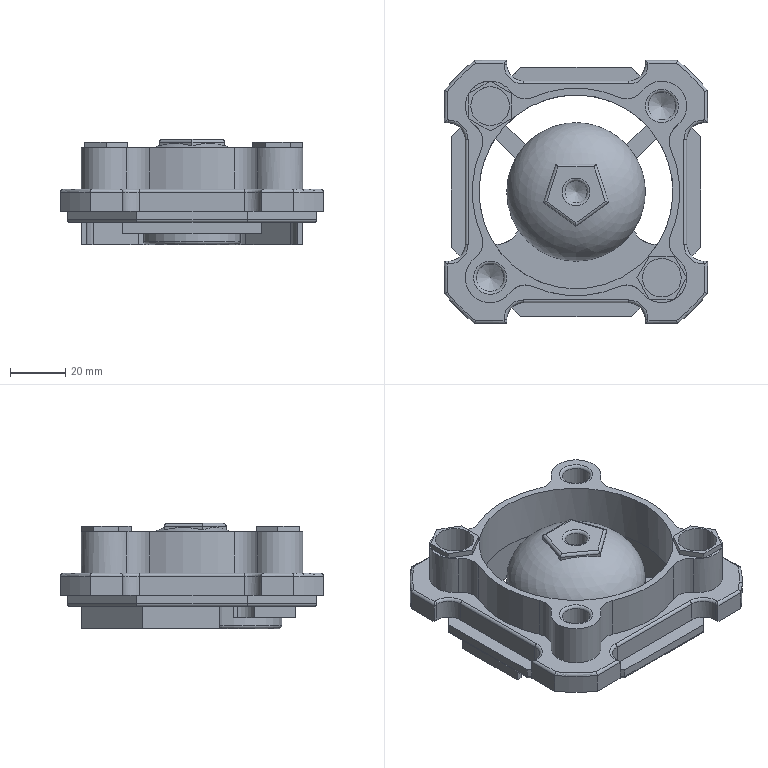NC program | NX | posted with a generic post | part box 95 x 95 x 38 mm
Lines 2303 to 3620 of 59038:
(FIXED_CONTOUR , TOOL : D4)
N4562 M6
N4564 G54
N4566 G17 G0 G90 X-12.931 Y-5.438 S3000 M3
N4568 G43 Z10. H0
N4570 Z3.6
N4572 G94 G1 Z-1. F2500.
N4574 X-1.176 Y-13.979
N4576 X-0.618 Y-14.263
N4578 X0. Y-14.361
N4580 X0.618 Y-14.263
N4582 X1.176 Y-13.979
N4584 X12.931 Y-5.438
N4586 X13.374 Y-4.995
N4588 X13.658 Y-4.438
N4590 X13.756 Y-3.82
N4592 X13.658 Y-3.202
N4594 X9.168 Y10.618
N4596 X8.883 Y11.176
N4598 X8.441 Y11.618
N4600 X7.883 Y11.902
N4602 X7.265 Y12.
N4604 X-7.265
N4606 X-7.883 Y11.902
N4608 X-8.441 Y11.618
N4610 X-8.883 Y11.176
N4612 X-9.168 Y10.618
N4614 X-13.658 Y-3.202
N4616 X-13.756 Y-3.82
N4618 X-13.658 Y-4.438
N4620 X-13.374 Y-4.995
N4622 X-12.931 Y-5.438
N4624 X-4.114 Y-11.844 Z-1.008
N4626 X-2.645 Y-12.911 Z-1.013
N4628 X-1.176 Y-13.979 Z-1.02
N4630 X-0.618 Y-14.263
N4632 X0. Y-14.361
N4634 X0.618 Y-14.263
N4636 X1.176 Y-13.979
N4638 X7.053 Y-9.708 Z-1.011
N4640 X11.462 Y-6.505 Z-1.027
N4642 X12.931 Y-5.438 Z-1.04
N4644 X13.374 Y-4.995
N4646 X13.658 Y-4.438
N4648 X13.756 Y-3.82
N4650 X13.658 Y-3.202
N4652 X11.974 Y1.98 Z-1.019
N4654 X11.413 Y3.708
N4656 X10.851 Y5.436 Z-1.022
N4658 X10.29 Y7.164 Z-1.029
N4660 X9.729 Y8.891 Z-1.042
N4662 X9.168 Y10.618 Z-1.06
N4664 X8.883 Y11.176
N4666 X8.441 Y11.618
N4668 X7.883 Y11.902
N4670 X7.265 Y12.
N4672 X5.45 Z-1.045
N4674 X3.634 Z-1.034
N4676 X1.817 Z-1.028
N4678 X0. Z-1.026
N4680 X-1.817 Z-1.03
N4682 X-3.634 Z-1.04
N4684 X-5.45 Z-1.056
N4686 X-7.265 Z-1.08
N4688 X-7.883 Y11.902
N4690 X-8.441 Y11.618
N4692 X-8.883 Y11.176
N4694 X-9.168 Y10.618
N4696 X-9.728 Y8.892 Z-1.06
N4698 X-10.29 Y7.165 Z-1.045
N4700 X-10.851 Y5.437 Z-1.036
N4702 X-11.413 Y3.708 Z-1.033
N4704 X-11.974 Y1.98 Z-1.038
N4706 X-12.536 Y0.251 Z-1.05
N4708 X-13.097 Y-1.476 Z-1.071
N4710 X-13.658 Y-3.202 Z-1.1
N4712 X-13.756 Y-3.82
N4714 X-13.658 Y-4.438
N4716 X-13.374 Y-4.995
N4718 X-12.931 Y-5.438
N4720 X-11.463 Y-6.504 Z-1.074
N4722 X-9.994 Y-7.572 Z-1.055
N4724 X-8.524 Y-8.64 Z-1.044
N4726 X-7.054 Y-9.708 Z-1.041
N4728 X-5.583 Y-10.776 Z-1.046
N4730 X-4.113 Y-11.845 Z-1.061
N4732 X-2.643 Y-12.912 Z-1.085
N4734 X-1.176 Y-13.979 Z-1.12
N4736 X-0.618 Y-14.263
N4738 X0. Y-14.361
N4740 X0.618 Y-14.263
N4742 X1.176 Y-13.979
N4744 X2.643 Y-12.912 Z-1.089
N4746 X4.113 Y-11.845 Z-1.066
N4748 X5.583 Y-10.777 Z-1.052
N4750 X7.053 Y-9.708 Z-1.048
N4752 X8.524 Y-8.64 Z-1.054
N4754 X9.995 Y-7.571 Z-1.071
N4756 X11.464 Y-6.504 Z-1.1
N4758 X12.931 Y-5.438 Z-1.14
N4760 X13.374 Y-4.995
N4762 X13.658 Y-4.438
N4764 X13.756 Y-3.82
N4766 X13.658 Y-3.202
N4768 X13.097 Y-1.476 Z-1.103
N4770 X12.536 Y0.251 Z-1.076
N4772 X11.974 Y1.979 Z-1.061
N4774 X11.413 Y3.708 Z-1.056
N4776 X10.851 Y5.437 Z-1.063
N4778 X10.289 Y7.166 Z-1.082
N4780 X9.728 Y8.893 Z-1.114
N4782 X9.168 Y10.618 Z-1.16
N4784 X8.883 Y11.176
N4786 X8.441 Y11.618
N4788 X7.883 Y11.902
N4790 X7.265 Y12.
N4792 X5.452 Z-1.118
N4794 X3.636 Z-1.087
N4796 X1.818 Z-1.069
N4798 X0. Z-1.063
N4800 X-1.818 Z-1.071
N4802 X-3.636 Z-1.092
N4804 X-5.452 Z-1.128
N4806 X-7.265 Z-1.18
N4808 X-7.883 Y11.902
N4810 X-8.441 Y11.618
N4812 X-8.883 Y11.176
N4814 X-9.168 Y10.618
N4816 X-9.728 Y8.893 Z-1.132
N4818 X-10.289 Y7.166 Z-1.098
N4820 X-10.851 Y5.438 Z-1.077
N4822 X-11.413 Y3.708 Z-1.071
N4824 X-11.974 Y1.979 Z-1.079
N4826 X-12.537 Y0.249 Z-1.103
N4828 X-13.098 Y-1.477 Z-1.143
N4830 X-13.658 Y-3.202 Z-1.2
N4832 X-13.756 Y-3.82
N4834 X-13.658 Y-4.438
N4836 X-13.374 Y-4.995
N4838 X-12.931 Y-5.438
N4840 X-11.465 Y-6.503 Z-1.147
N4842 X-9.995 Y-7.571 Z-1.108
N4844 X-8.525 Y-8.639 Z-1.085
N4846 X-7.054 Y-9.708 Z-1.078
N4848 X-5.582 Y-10.777 Z-1.087
N4850 X-4.111 Y-11.846 Z-1.113
N4852 X-2.642 Y-12.913 Z-1.157
N4854 X-1.176 Y-13.979 Z-1.22
N4856 X-0.618 Y-14.263
N4858 X0. Y-14.361
N4860 X0.618 Y-14.263
N4862 X1.176 Y-13.979
N4864 X2.642 Y-12.913 Z-1.161
N4866 X4.111 Y-11.846 Z-1.119
N4868 X5.582 Y-10.777 Z-1.093
N4870 X7.053 Y-9.708 Z-1.085
N4872 X8.525 Y-8.639 Z-1.095
N4874 X9.996 Y-7.57 Z-1.124
N4876 X11.465 Y-6.503 Z-1.172
N4878 X12.931 Y-5.438 Z-1.24
N4880 X13.374 Y-4.995
N4882 X13.658 Y-4.438
N4884 X13.756 Y-3.82
N4886 X13.658 Y-3.202
N4888 X13.098 Y-1.478 Z-1.176
N4890 X12.537 Y0.249 Z-1.129
N4892 X11.975 Y1.978 Z-1.102
N4894 X11.413 Y3.708 Z-1.093
N4896 X10.851 Y5.438 Z-1.104
N4898 X10.288 Y7.168 Z-1.135
N4900 X9.728 Y8.895 Z-1.186
N4902 X9.168 Y10.618 Z-1.26
N4904 X8.883 Y11.176
N4906 X8.441 Y11.618
N4908 X7.883 Y11.902
N4910 X7.265 Y12.
N4912 X5.453 Z-1.19
N4914 X3.637 Z-1.14
N4916 X1.819 Z-1.11
N4918 X0. Z-1.1
N4920 X-1.819 Z-1.112
N4922 X-3.639 Z-1.145
N4924 X-5.454 Z-1.201
N4926 X-7.265 Z-1.28
N4928 X-7.883 Y11.902
N4930 X-8.441 Y11.618
N4932 X-8.883 Y11.176
N4934 X-9.168 Y10.618
N4936 X-9.727 Y8.895 Z-1.204
N4938 X-10.289 Y7.168 Z-1.15
N4940 X-10.85 Y5.439 Z-1.118
N4942 X-11.413 Y3.709 Z-1.108
N4944 X-11.975 Y1.978 Z-1.12
N4946 X-12.537 Y0.247 Z-1.156
N4948 X-13.098 Y-1.479 Z-1.215
N4950 X-13.658 Y-3.202 Z-1.3
N4952 X-13.756 Y-3.82
N4954 X-13.658 Y-4.438
N4956 X-13.374 Y-4.995
N4958 X-12.931 Y-5.438
N4960 X-11.466 Y-6.502 Z-1.219
N4962 X-9.997 Y-7.57 Z-1.161
N4964 X-8.526 Y-8.639 Z-1.126
N4966 X-7.054 Y-9.708 Z-1.115
N4968 X-5.582 Y-10.777 Z-1.128
N4970 X-4.109 Y-11.847 Z-1.166
N4972 X-2.641 Y-12.914 Z-1.23
N4974 X-1.176 Y-13.979 Z-1.32
N4976 X-0.618 Y-14.263
N4978 X0. Y-14.361
N4980 X0.618 Y-14.263
N4982 X1.176 Y-13.979
N4984 X2.641 Y-12.914 Z-1.233
N4986 X4.11 Y-11.847 Z-1.171
N4988 X5.581 Y-10.778 Z-1.134
N4990 X7.053 Y-9.708 Z-1.123
N4992 X8.525 Y-8.639 Z-1.136
N4994 X9.998 Y-7.569 Z-1.177
N4996 X11.466 Y-6.502 Z-1.244
N4998 X12.931 Y-5.438 Z-1.34
N5000 X13.374 Y-4.995
N5002 X13.658 Y-4.438
N5004 X13.756 Y-3.82
N5006 X13.658 Y-3.202
N5008 X13.098 Y-1.48 Z-1.248
N5010 X12.537 Y0.248 Z-1.182
N5012 X11.975 Y1.977 Z-1.143
N5014 X11.413 Y3.708 Z-1.13
N5016 X10.85 Y5.439 Z-1.145
N5018 X10.288 Y7.17 Z-1.187
N5020 X9.727 Y8.896 Z-1.259
N5022 X9.168 Y10.618 Z-1.36
N5024 X8.883 Y11.176
N5026 X8.441 Y11.618
N5028 X7.883 Y11.902
N5030 X7.265 Y12.
N5032 X5.455 Z-1.262
N5034 X3.639 Z-1.192
N5036 X1.82 Z-1.151
N5038 X0.001 Z-1.137
N5040 X-1.82 Z-1.153
N5042 X-3.641 Z-1.198
N5044 X-5.455 Z-1.273
N5046 X-7.265 Z-1.38
N5048 X-7.883 Y11.902
N5050 X-8.441 Y11.618
N5052 X-8.883 Y11.176
N5054 X-9.168 Y10.618
N5056 X-9.727 Y8.897 Z-1.277
N5058 X-10.288 Y7.169 Z-1.203
N5060 X-10.85 Y5.44 Z-1.159
N5062 X-11.413 Y3.709 Z-1.145
N5064 X-11.975 Y1.977 Z-1.161
N5066 X-12.538 Y0.245 Z-1.208
N5068 X-13.099 Y-1.48 Z-1.288
N5070 X-13.658 Y-3.202 Z-1.4
N5072 X-13.756 Y-3.82
N5074 X-13.658 Y-4.438
N5076 X-13.374 Y-4.995
N5078 X-12.931 Y-5.438
N5080 X-11.467 Y-6.501 Z-1.291
N5082 X-9.998 Y-7.569 Z-1.214
N5084 X-8.527 Y-8.638 Z-1.167
N5086 X-7.054 Y-9.708 Z-1.152
N5088 X-5.581 Y-10.778 Z-1.169
N5090 X-4.107 Y-11.849 Z-1.219
N5092 X-2.639 Y-12.915 Z-1.302
N5094 X-1.176 Y-13.979 Z-1.42
N5096 X-0.618 Y-14.263
N5098 X0. Y-14.361
N5100 X0.618 Y-14.263
N5102 X1.176 Y-13.979
N5104 X2.639 Y-12.915 Z-1.306
N5106 X4.109 Y-11.848 Z-1.224
N5108 X5.58 Y-10.779 Z-1.175
N5110 X7.053 Y-9.709 Z-1.16
N5112 X8.526 Y-8.638 Z-1.177
N5114 X10. Y-7.568 Z-1.23
N5116 X11.468 Y-6.501 Z-1.317
N5118 X12.931 Y-5.438 Z-1.44
N5120 X13.374 Y-4.995
N5122 X13.658 Y-4.438
N5124 X13.756 Y-3.82
N5126 X13.658 Y-3.202
N5128 X13.099 Y-1.481 Z-1.32
N5130 X12.538 Y0.246 Z-1.235
N5132 X11.976 Y1.976 Z-1.184
N5134 X11.413 Y3.708 Z-1.167
N5136 X10.85 Y5.439 Z-1.186
N5138 X10.287 Y7.172 Z-1.24
N5140 X9.727 Y8.898 Z-1.331
N5142 X9.168 Y10.618 Z-1.46
N5144 X8.883 Y11.176
N5146 X8.441 Y11.618
N5148 X7.883 Y11.902
N5150 X7.265 Y12.
N5152 X5.457 Z-1.335
N5154 X3.641 Z-1.245
N5156 X1.822 Z-1.192
N5158 X0.001 Z-1.175
N5160 X-1.821 Z-1.194
N5162 X-3.643 Z-1.251
N5164 X-5.457 Z-1.346
N5166 X-7.265 Z-1.48
N5168 X-7.883 Y11.902
N5170 X-8.441 Y11.618
N5172 X-8.883 Y11.176
N5174 X-9.168 Y10.618
N5176 X-9.726 Y8.898 Z-1.349
N5178 X-10.288 Y7.171 Z-1.256
N5180 X-10.85 Y5.441 Z-1.2
N5182 X-11.412 Y3.709 Z-1.182
N5184 X-11.975 Y1.977 Z-1.202
N5186 X-12.538 Y0.243 Z-1.261
N5188 X-13.099 Y-1.482 Z-1.36
N5190 X-13.658 Y-3.202 Z-1.5
N5192 X-13.756 Y-3.82
N5194 X-13.658 Y-4.438
N5196 X-13.374 Y-4.995
N5198 X-12.931 Y-5.438
N5200 X-11.469 Y-6.5 Z-1.364
N5202 X-9.999 Y-7.568 Z-1.266
N5204 X-8.527 Y-8.637 Z-1.208
N5206 X-7.054 Y-9.708 Z-1.189
N5208 X-5.58 Y-10.778 Z-1.21
N5210 X-4.106 Y-11.85 Z-1.272
N5212 X-2.638 Y-12.916 Z-1.374
N5214 X-1.176 Y-13.979 Z-1.52
N5216 X-0.618 Y-14.263
N5218 X0. Y-14.361
N5220 X0.618 Y-14.263
N5222 X1.176 Y-13.979
N5224 X2.638 Y-12.916 Z-1.378
N5226 X4.107 Y-11.849 Z-1.277
N5228 X5.579 Y-10.779 Z-1.216
N5230 X7.053 Y-9.709 Z-1.197
N5232 X8.527 Y-8.638 Z-1.218
N5234 X10.001 Y-7.566 Z-1.282
N5236 X11.469 Y-6.5 Z-1.389
N5238 X12.931 Y-5.438 Z-1.54
N5240 X13.374 Y-4.995
N5242 X13.658 Y-4.438
N5244 X13.756 Y-3.82
N5246 X13.658 Y-3.202
N5248 X13.099 Y-1.483 Z-1.393
N5250 X12.538 Y0.244 Z-1.287
N5252 X11.976 Y1.975 Z-1.225
N5254 X11.413 Y3.707 Z-1.204
N5256 X10.85 Y5.44 Z-1.227
N5258 X10.286 Y7.174 Z-1.293
N5260 X9.726 Y8.899 Z-1.403
N5262 X9.168 Y10.618 Z-1.56
N5264 X8.883 Y11.176
N5266 X8.441 Y11.618
N5268 X7.883 Y11.902
N5270 X7.265 Y12.
N5272 X5.459 Z-1.407
N5274 X3.642 Z-1.298
N5276 X1.823 Z-1.233
N5278 X0.001 Z-1.212
N5280 X-1.821 Z-1.235
N5282 X-3.645 Z-1.303
N5284 X-5.459 Z-1.418
N5286 X-7.265 Z-1.58
N5288 X-7.883 Y11.902
N5290 X-8.441 Y11.618
N5292 X-8.883 Y11.176
N5294 X-9.168 Y10.618
N5296 X-9.726 Y8.9 Z-1.422
N5298 X-10.287 Y7.173 Z-1.309
N5300 X-10.849 Y5.442 Z-1.241
N5302 X-11.412 Y3.709 Z-1.219
N5304 X-11.976 Y1.976 Z-1.243
N5306 X-12.539 Y0.241 Z-1.314
N5308 X-13.1 Y-1.483 Z-1.432
N5310 X-13.658 Y-3.202 Z-1.6
N5312 X-13.756 Y-3.82
N5314 X-13.658 Y-4.438
N5316 X-13.374 Y-4.995
N5318 X-12.931 Y-5.438
N5320 X-11.47 Y-6.499 Z-1.436
N5322 X-10.001 Y-7.567 Z-1.319
N5324 X-8.528 Y-8.637 Z-1.249
N5326 X-7.054 Y-9.708 Z-1.226
N5328 X-5.58 Y-10.779 Z-1.251
N5330 X-4.104 Y-11.851 Z-1.325
N5332 X-2.637 Y-12.917 Z-1.447
N5334 X-1.176 Y-13.979 Z-1.62
N5336 X-0.618 Y-14.263
N5338 X0. Y-14.361
N5340 X0.618 Y-14.263
N5342 X1.176 Y-13.979
N5344 X2.637 Y-12.917 Z-1.451
N5346 X4.106 Y-11.85 Z-1.33
N5348 X5.578 Y-10.78 Z-1.257
N5350 X7.053 Y-9.709 Z-1.234
N5352 X8.527 Y-8.637 Z-1.259
N5354 X10.003 Y-7.565 Z-1.335
N5356 X11.47 Y-6.499 Z-1.461
N5358 X12.931 Y-5.438 Z-1.64
N5360 X13.374 Y-4.995
N5362 X13.658 Y-4.438
N5364 X13.756 Y-3.82
N5366 X13.658 Y-3.202
N5368 X13.1 Y-1.484 Z-1.465
N5370 X12.539 Y0.243 Z-1.34
N5372 X11.976 Y1.974 Z-1.266
N5374 X11.413 Y3.707 Z-1.241
N5376 X10.85 Y5.441 Z-1.268
N5378 X10.286 Y7.176 Z-1.346
N5380 X9.725 Y8.901 Z-1.476
N5382 X9.168 Y10.618 Z-1.66
N5384 X8.883 Y11.176
N5386 X8.441 Y11.618
N5388 X7.883 Y11.902
N5390 X7.265 Y12.
N5392 X5.46 Z-1.479
N5394 X3.644 Z-1.351
N5396 X1.824 Z-1.274
N5398 X0.001 Z-1.249
N5400 X-1.822 Z-1.276
N5402 X-3.647 Z-1.356
N5404 X-5.46 Z-1.49
N5406 X-7.265 Z-1.68
N5408 X-7.883 Y11.902
N5410 X-8.441 Y11.618
N5412 X-8.883 Y11.176
N5414 X-9.168 Y10.618
N5416 X-9.725 Y8.901 Z-1.494
N5418 X-10.286 Y7.174 Z-1.361
N5420 X-10.849 Y5.443 Z-1.282
N5422 X-11.412 Y3.709 Z-1.256
N5424 X-11.976 Y1.975 Z-1.284
N5426 X-12.54 Y0.239 Z-1.367
N5428 X-13.1 Y-1.485 Z-1.505
N5430 X-13.658 Y-3.202 Z-1.7
N5432 X-13.756 Y-3.82
N5434 X-13.658 Y-4.438
N5436 X-13.374 Y-4.995
N5438 X-12.931 Y-5.438
N5440 X-11.471 Y-6.498 Z-1.508
N5442 X-10.002 Y-7.566 Z-1.372
N5444 X-8.529 Y-8.636 Z-1.29
N5446 X-7.054 Y-9.708 Z-1.264
N5448 X-5.579 Y-10.78 Z-1.292
N5450 X-4.102 Y-11.852 Z-1.377
N5452 X-2.636 Y-12.918 Z-1.519
N5454 X-1.176 Y-13.979 Z-1.72
N5456 X-0.618 Y-14.263
N5458 X0. Y-14.361
N5460 X0.618 Y-14.263
N5462 X1.176 Y-13.979
N5464 X2.635 Y-12.918 Z-1.523
N5466 X4.104 Y-11.851 Z-1.382
N5468 X5.577 Y-10.781 Z-1.298
N5470 X7.053 Y-9.709 Z-1.271
N5472 X8.528 Y-8.637 Z-1.3
N5474 X10.005 Y-7.564 Z-1.388
N5476 X11.472 Y-6.498 Z-1.534
N5478 X12.931 Y-5.438 Z-1.74
N5480 X13.374 Y-4.995
N5482 X13.658 Y-4.438
N5484 X13.756 Y-3.82
N5486 X13.658 Y-3.202
N5488 X13.1 Y-1.486 Z-1.537
N5490 X12.539 Y0.241 Z-1.393
N5492 X11.977 Y1.973 Z-1.307
N5494 X11.413 Y3.707 Z-1.278
N5496 X10.849 Y5.442 Z-1.309
N5498 X10.285 Y7.178 Z-1.399
N5500 X9.725 Y8.902 Z-1.548
N5502 X9.168 Y10.618 Z-1.76
N5504 X8.883 Y11.176
N5506 X8.441 Y11.618
N5508 X7.883 Y11.902
N5510 X7.265 Y12.
N5512 X5.462 Z-1.552
N5514 X3.646 Z-1.403
N5516 X1.825 Z-1.315
N5518 X0.001 Z-1.286
N5520 X-1.823 Z-1.317
N5522 X-3.649 Z-1.409
N5524 X-5.462 Z-1.563
N5526 X-7.265 Z-1.78
N5528 X-7.883 Y11.902
N5530 X-8.441 Y11.618
N5532 X-8.883 Y11.176
N5534 X-9.168 Y10.618
N5536 X-9.725 Y8.903 Z-1.566
N5538 X-10.286 Y7.176 Z-1.414
N5540 X-10.849 Y5.444 Z-1.323
N5542 X-11.412 Y3.709 Z-1.293
N5544 X-11.976 Y1.974 Z-1.325
N5546 X-12.54 Y0.237 Z-1.42
N5548 X-13.101 Y-1.487 Z-1.577
N5550 X-13.658 Y-3.202 Z-1.8
N5552 X-13.756 Y-3.82
N5554 X-13.658 Y-4.438
N5556 X-13.374 Y-4.995
N5558 X-12.931 Y-5.438
N5560 X-11.473 Y-6.497 Z-1.581
N5562 X-10.004 Y-7.565 Z-1.425
N5564 X-8.53 Y-8.635 Z-1.331
N5566 X-7.054 Y-9.708 Z-1.301
N5568 X-5.578 Y-10.78 Z-1.333
N5570 X-4.101 Y-11.854 Z-1.43
N5572 X-2.634 Y-12.919 Z-1.592
N5574 X-1.176 Y-13.979 Z-1.82
N5576 X-0.618 Y-14.263
N5578 X0. Y-14.361
N5580 X0.618 Y-14.263
N5582 X1.176 Y-13.979
N5584 X2.634 Y-12.919 Z-1.595
N5586 X4.103 Y-11.852 Z-1.435
N5588 X5.576 Y-10.781 Z-1.339
N5590 X7.052 Y-9.709 Z-1.308
N5592 X8.529 Y-8.636 Z-1.341
N5594 X10.007 Y-7.563 Z-1.441
N5596 X11.473 Y-6.497 Z-1.606
N5598 X12.931 Y-5.438 Z-1.84
N5600 X13.374 Y-4.995
N5602 X13.658 Y-4.438
N5604 X13.756 Y-3.82
N5606 X13.658 Y-3.202
N5608 X13.101 Y-1.488 Z-1.61
N5610 X12.54 Y0.239 Z-1.446
N5612 X11.977 Y1.972 Z-1.348
N5614 X11.413 Y3.707 Z-1.316
N5616 X10.849 Y5.443 Z-1.35
N5618 X10.285 Y7.18 Z-1.451
N5620 X9.724 Y8.904 Z-1.621
N5622 X9.168 Y10.618 Z-1.86
N5624 X8.883 Y11.176
N5626 X8.441 Y11.618
N5628 X7.883 Y11.902
N5630 X7.265 Y12.
N5632 X5.464 Z-1.624
N5634 X3.648 Z-1.456
N5636 X1.826 Z-1.356
N5638 X0.001 Z-1.323
N5640 X-1.824 Z-1.358
N5642 X-3.651 Z-1.462
N5644 X-5.463 Z-1.635
N5646 X-7.265 Z-1.88
N5648 X-7.883 Y11.902
N5650 X-8.441 Y11.618
N5652 X-8.883 Y11.176
N5654 X-9.168 Y10.618
N5656 X-9.724 Y8.905 Z-1.639
N5658 X-10.285 Y7.178 Z-1.467
N5660 X-10.848 Y5.445 Z-1.364
N5662 X-11.412 Y3.709 Z-1.33
N5664 X-11.976 Y1.973 Z-1.366
N5666 X-12.541 Y0.235 Z-1.472
N5668 X-13.101 Y-1.488 Z-1.649
N5670 X-13.658 Y-3.202 Z-1.9
N5672 X-13.756 Y-3.82
N5674 X-13.658 Y-4.438
N5676 X-13.374 Y-4.995
N5678 X-12.931 Y-5.438
N5680 X-11.474 Y-6.496 Z-1.653
N5682 X-10.005 Y-7.564 Z-1.477
N5684 X-8.531 Y-8.635 Z-1.372
N5686 X-7.054 Y-9.707 Z-1.338
N5688 X-5.577 Y-10.781 Z-1.374
N5690 X-4.099 Y-11.855 Z-1.483
N5692 X-2.633 Y-12.92 Z-1.664
N5694 X-1.176 Y-13.979 Z-1.92
N5696 X-0.618 Y-14.263
N5698 X0. Y-14.361
N5700 X0.618 Y-14.263
N5702 X1.176 Y-13.979
N5704 X2.632 Y-12.92 Z-1.668
N5706 X4.102 Y-11.853 Z-1.488
N5708 X5.576 Y-10.782 Z-1.38
N5710 X7.052 Y-9.709 Z-1.345
N5712 X8.53 Y-8.636 Z-1.382
N5714 X10.008 Y-7.561 Z-1.494
N5716 X11.474 Y-6.496 Z-1.678
N5718 X12.931 Y-5.438 Z-1.94
N5720 X13.374 Y-4.995
N5722 X13.658 Y-4.438
N5724 X13.756 Y-3.82
N5726 X13.658 Y-3.202
N5728 X13.101 Y-1.489 Z-1.682
N5730 X12.54 Y0.238 Z-1.498
N5732 X11.977 Y1.971 Z-1.389
N5734 X11.413 Y3.707 Z-1.353
N5736 X10.849 Y5.444 Z-1.391
N5738 X10.284 Y7.182 Z-1.504
N5740 X9.724 Y8.906 Z-1.693
N5742 X9.445 Y9.764 Z-1.817
N5744 X9.168 Y10.618 Z-1.96
N5746 X8.883 Y11.176
N5748 X8.441 Y11.618
N5750 X7.883 Y11.902
N5752 X7.265 Y12.
N5754 X5.465 Z-1.697
N5756 X3.649 Z-1.509
N5758 X1.827 Z-1.397
N5760 X0.001 Z-1.36
N5762 X-1.825 Z-1.399
N5764 X-3.653 Z-1.515
N5766 X-5.465 Z-1.707
N5768 X-6.367 Z-1.834
N5770 X-7.265 Z-1.98
N5772 X-7.883 Y11.902
N5774 X-8.441 Y11.618
N5776 X-8.883 Y11.176
N5778 X-9.168 Y10.618
N5780 X-9.724 Y8.906 Z-1.711
N5782 X-10.285 Y7.179 Z-1.519
N5784 X-10.848 Y5.446 Z-1.405
N5786 X-11.412 Y3.71 Z-1.368
N5788 X-11.977 Y1.972 Z-1.407
N5790 X-12.542 Y0.233 Z-1.525
N5792 X-12.822 Y-0.63 Z-1.614
N5794 X-13.102 Y-1.49 Z-1.722
N5796 X-13.38 Y-2.348 Z-1.851
N5798 X-13.658 Y-3.202 Z-2.
N5800 X-13.756 Y-3.82
N5802 X-13.658 Y-4.438
N5804 X-13.374 Y-4.995
N5806 X-12.931 Y-5.438
N5808 X-12.204 Y-5.966 Z-1.853
N5810 X-11.475 Y-6.495 Z-1.726
N5812 X-10.006 Y-7.563 Z-1.53
N5814 X-8.532 Y-8.634 Z-1.413
N5816 X-7.055 Y-9.707 Z-1.375
N5818 X-5.577 Y-10.781 Z-1.415
N5820 X-4.836 Y-11.319 Z-1.465
N5822 X-4.097 Y-11.856 Z-1.536
N5824 X-3.363 Y-12.389 Z-1.626
N5826 X-2.632 Y-12.921 Z-1.736
N5828 X-1.902 Y-13.451 Z-1.868
N5830 X-1.176 Y-13.979 Z-2.02
N5832 X-0.618 Y-14.263
N5834 X0. Y-14.361
N5836 X0.618 Y-14.263
N5838 X1.176 Y-13.979
N5840 X1.903 Y-13.451 Z-1.87
N5842 X2.631 Y-12.921 Z-1.74
N5844 X3.365 Y-12.388 Z-1.63
N5846 X4.1 Y-11.854 Z-1.541
N5848 X4.837 Y-11.319 Z-1.471
N5850 X5.575 Y-10.783 Z-1.421
N5852 X7.052 Y-9.709 Z-1.382
N5854 X7.791 Y-9.172 Z-1.393
N5856 X8.53 Y-8.635 Z-1.423
N5858 X9.271 Y-8.097 Z-1.475
N5860 X10.01 Y-7.56 Z-1.546
N5862 X10.744 Y-7.027 Z-1.638
N5864 X11.476 Y-6.495 Z-1.751
N5866 X12.205 Y-5.965 Z-1.885
N5868 X12.931 Y-5.438 Z-2.04
N5870 X13.374 Y-4.995
N5872 X13.658 Y-4.438
N5874 X13.756 Y-3.82
N5876 X13.658 Y-3.202
N5878 X13.38 Y-2.347 Z-1.887
N5880 X13.102 Y-1.491 Z-1.754
N5882 X12.822 Y-0.629 Z-1.642
N5884 X12.541 Y0.236 Z-1.551
N5886 X12.259 Y1.102 Z-1.48
N5888 X11.978 Y1.97 Z-1.43
N5890 X11.695 Y2.838 Z-1.4
N5892 X11.413 Y3.707 Z-1.39
N5894 X11.131 Y4.575 Z-1.4
N5896 X10.849 Y5.445 Z-1.432
N5898 X10.565 Y6.316 Z-1.484
N5900 X10.283 Y7.184 Z-1.557
N5902 X10.003 Y8.047 Z-1.65
N5904 X9.723 Y8.907 Z-1.765
N5906 X9.445 Y9.764 Z-1.902
N5908 X9.168 Y10.618 Z-2.06
N5910 X8.883 Y11.176
N5912 X8.441 Y11.618
N5914 X7.883 Y11.902
N5916 X7.265 Y12.
N5918 X6.367 Z-1.904
N5920 X5.467 Z-1.769
N5922 X4.56 Z-1.655
N5924 X3.651 Z-1.562
N5926 X2.74 Z-1.489
N5928 X1.828 Z-1.438
N5930 X0.915 Z-1.407
N5932 X0.002 Z-1.397
N5934 X-0.912 Z-1.408
N5936 X-1.826 Z-1.44
N5938 X-2.742 Z-1.493
N5940 X-3.655 Z-1.567
N5942 X-4.563 Z-1.663
N5944 X-5.467 Z-1.78
N5946 X-6.368 Z-1.919
N5948 X-7.265 Z-2.08
N5950 X-7.883 Y11.902
N5952 X-8.441 Y11.618
N5954 X-8.883 Y11.176
N5956 X-9.168 Y10.618
N5958 X-9.445 Y9.764 Z-1.921
N5960 X-9.723 Y8.908 Z-1.783
N5962 X-10.003 Y8.046 Z-1.667
N5964 X-10.284 Y7.181 Z-1.572
N5966 X-10.566 Y6.315 Z-1.499
N5968 X-10.848 Y5.447 Z-1.446
N5970 X-11.13 Y4.578 Z-1.415
N5972 X-11.412 Y3.71 Z-1.405
N5974 X-11.694 Y2.841 Z-1.416
N5976 X-11.977 Y1.972 Z-1.448
N5978 X-12.26 Y1.1 Z-1.502
N5980 X-12.542 Y0.231 Z-1.578
N5982 X-12.823 Y-0.631 Z-1.675
N5984 X-13.102 Y-1.491 Z-1.794
N5986 X-13.381 Y-2.348 Z-1.936
N5988 X-13.658 Y-3.202 Z-2.1
N5990 X-13.756 Y-3.82
N5992 X-13.658 Y-4.438
N5994 X-13.374 Y-4.995
N5996 X-12.931 Y-5.438
N5998 X-12.205 Y-5.965 Z-1.938
N6000 X-11.477 Y-6.494 Z-1.798
N6002 X-10.743 Y-7.027 Z-1.679
N6004 X-10.008 Y-7.562 Z-1.583
N6006 X-9.271 Y-8.097 Z-1.508
N6008 X-8.533 Y-8.633 Z-1.454
N6010 X-7.794 Y-9.17 Z-1.422
N6012 X-7.055 Y-9.707 Z-1.412
N6014 X-6.316 Y-10.244 Z-1.423
N6016 X-5.576 Y-10.782 Z-1.456
N6018 X-4.834 Y-11.32 Z-1.511
N6020 X-4.095 Y-11.857 Z-1.589
N6022 X-3.362 Y-12.391 Z-1.687
N6024 X-2.63 Y-12.922 Z-1.809
N6026 X-1.901 Y-13.452 Z-1.953
N6028 X-1.176 Y-13.979 Z-2.12
N6030 X-0.618 Y-14.263
N6032 X0. Y-14.361
N6034 X0.618 Y-14.263
N6036 X1.176 Y-13.979
N6038 X1.902 Y-13.451 Z-1.955
N6040 X2.63 Y-12.922 Z-1.812
N6042 X3.363 Y-12.389 Z-1.692
N6044 X4.099 Y-11.855 Z-1.593
N6046 X4.836 Y-11.319 Z-1.517
N6048 X5.574 Y-10.783 Z-1.462
N6050 X6.313 Y-10.246 Z-1.43
N6052 X7.052 Y-9.709 Z-1.42
N6054 X7.791 Y-9.172 Z-1.431
N6056 X8.531 Y-8.635 Z-1.464
N6058 X9.273 Y-8.096 Z-1.521
N6060 X10.012 Y-7.559 Z-1.599
N6062 X10.746 Y-7.026 Z-1.7
N6064 X11.477 Y-6.494 Z-1.823
N6066 X12.206 Y-5.965 Z-1.97
N6068 X12.931 Y-5.438 Z-2.14
N6070 X13.374 Y-4.995
N6072 X13.658 Y-4.438
N6074 X13.756 Y-3.82
N6076 X13.658 Y-3.202
N6078 X13.381 Y-2.348 Z-1.972
N6080 X13.102 Y-1.492 Z-1.827
N6082 X12.822 Y-0.63 Z-1.704
N6084 X12.541 Y0.235 Z-1.604
N6086 X12.26 Y1.101 Z-1.526
N6088 X11.978 Y1.969 Z-1.471
N6090 X11.696 Y2.838 Z-1.438
N6092 X11.413 Y3.707 Z-1.427
N6094 X11.131 Y4.576 Z-1.439
N6096 X10.848 Y5.445 Z-1.473
N6098 X10.565 Y6.317 Z-1.53
N6100 X10.283 Y7.186 Z-1.61
N6102 X10.002 Y8.049 Z-1.712
N6104 X9.723 Y8.909 Z-1.838
N6106 X9.445 Y9.765 Z-1.987
N6108 X9.168 Y10.618 Z-2.16
N6110 X8.883 Y11.176
N6112 X8.441 Y11.618
N6114 X7.883 Y11.902
N6116 X7.265 Y12.
N6118 X6.368 Z-1.989
N6120 X5.469 Z-1.841
N6122 X4.562 Z-1.716
N6124 X3.653 Z-1.614
N6126 X2.742 Z-1.535
N6128 X1.829 Z-1.479
N6130 X0.915 Z-1.445
N6132 X0.002 Z-1.434
N6134 X-0.912 Z-1.446
N6136 X-1.827 Z-1.481
N6138 X-2.744 Z-1.539
N6140 X-3.657 Z-1.62
N6142 X-4.565 Z-1.724
N6144 X-5.468 Z-1.852
N6146 X-6.369 Z-2.004
N6148 X-7.265 Z-2.18
N6150 X-7.883 Y11.902
N6152 X-8.441 Y11.618
N6154 X-8.883 Y11.176
N6156 X-9.168 Y10.618
N6158 X-9.445 Y9.765 Z-2.006
N6160 X-9.723 Y8.909 Z-1.856
N6162 X-10.003 Y8.047 Z-1.729
N6164 X-10.284 Y7.183 Z-1.625
N6166 X-10.565 Y6.316 Z-1.544
N6168 X-10.847 Y5.448 Z-1.487
N6170 X-11.13 Y4.579 Z-1.453
N6172 X-11.412 Y3.71 Z-1.442
N6174 X-11.695 Y2.841 Z-1.454
N6176 X-11.977 Y1.971 Z-1.489
N6178 X-12.261 Y1.098 Z-1.548
N6180 X-12.543 Y0.229 Z-1.631
N6182 X-12.823 Y-0.633 Z-1.737
N6184 X-13.103 Y-1.493 Z-1.867
N6186 X-13.381 Y-2.349 Z-2.021
N6188 X-13.658 Y-3.202 Z-2.2
N6190 X-13.756 Y-3.82
N6192 X-13.658 Y-4.438
N6194 X-13.374 Y-4.995
N6196 X-12.931 Y-5.438
N6198 X-12.206 Y-5.965 Z-2.023
N6200 X-11.478 Y-6.493 Z-1.87
N6202 X-10.745 Y-7.026 Z-1.741
N6204 X-10.009 Y-7.561 Z-1.635
N6206 X-9.272 Y-8.096 Z-1.554
N6208 X-8.534 Y-8.633 Z-1.495
N6210 X-7.794 Y-9.17 Z-1.461
N6212 X-7.055 Y-9.707 Z-1.449
N6214 X-6.315 Y-10.244 Z-1.461
N6216 X-5.575 Y-10.782 Z-1.497
N6218 X-4.833 Y-11.321 Z-1.557
N6220 X-4.094 Y-11.859 Z-1.641
N6222 X-3.36 Y-12.392 Z-1.749
N6224 X-2.629 Y-12.923 Z-1.881
N6226 X-1.9 Y-13.452 Z-2.038
N6228 X-1.176 Y-13.979 Z-2.22
N6230 X-0.618 Y-14.263
N6232 X0. Y-14.361
N6234 X0.618 Y-14.263
N6236 X1.176 Y-13.979
N6238 X1.901 Y-13.452 Z-2.04
N6240 X2.628 Y-12.923 Z-1.885
N6242 X3.362 Y-12.39 Z-1.753
N6244 X4.097 Y-11.856 Z-1.646
N6246 X4.834 Y-11.32 Z-1.563
N6248 X5.573 Y-10.784 Z-1.504
N6250 X6.312 Y-10.247 Z-1.468
N6252 X7.052 Y-9.709 Z-1.457
N6254 X7.791 Y-9.172 Z-1.469
N6256 X8.532 Y-8.634 Z-1.505
N6258 X9.274 Y-8.095 Z-1.566
N6260 X10.013 Y-7.558 Z-1.652
N6262 X10.747 Y-7.024 Z-1.761
N6264 X11.478 Y-6.493 Z-1.896
N6266 X11.875 Y-6.205 Z-1.979
N6268 X12.216 Y-5.977 Z-2.055
N6270 X12.966 Y-5.485 Z-2.24
N6272 X13.011 Y-5.377
N6274 X13.403 Y-4.954
N6276 X13.658 Y-4.438
N6278 X13.755 Y-3.87
N6280 X13.686 Y-3.297
N6282 X13.713 Y-3.184
N6284 X13.402 Y-2.342 Z-2.057
N6286 X13.184 Y-1.742 Z-1.942
N6288 X13.103 Y-1.494 Z-1.899
N6290 X12.823 Y-0.632 Z-1.766
N6292 X12.542 Y0.233 Z-1.657
N6294 X12.26 Y1.099 Z-1.572
N6296 X11.978 Y1.967 Z-1.512
N6298 X11.696 Y2.837 Z-1.476
N6300 X11.413 Y3.707 Z-1.464
N6302 X11.131 Y4.576 Z-1.477
N6304 X10.848 Y5.446 Z-1.514
N6306 X10.564 Y6.319 Z-1.576
N6308 X10.282 Y7.188 Z-1.662
N6310 X10.002 Y8.051 Z-1.774
N6312 X9.862 Y8.481 Z-1.839
N6314 X9.743 Y8.917 Z-1.91
N6316 X9.508 Y9.787 Z-2.072
N6318 X9.279 Y10.654 Z-2.26
N6320 X9.093 Y10.813
N6322 X8.82 Y11.259
N6324 X8.441 Y11.618
N6326 X7.982 Y11.867
N6328 X7.474 Y11.989
N6330 X7.265 Y12.117
N6332 X6.369 Y12.073 Z-2.074
N6334 X5.47 Y12.032 Z-1.914
N6336 X4.665 Y12. Z-1.792
N6338 X4.564 Z-1.778
N6340 X3.654 Z-1.667
N6342 X2.743 Z-1.581
N6344 X1.831 Z-1.52
N6346 X0.916 Z-1.483
N6348 X0.002 Z-1.472
N6350 X-0.912 Z-1.484
N6352 X-1.828 Z-1.522
N6354 X-2.745 Z-1.585
N6356 X-3.66 Z-1.673
N6358 X-4.114 Z-1.726
N6360 X-4.567 Y12.019 Z-1.786
N6362 X-5.47 Y12.065 Z-1.924
N6364 X-6.37 Y12.118 Z-2.089
N6366 X-7.265 Y12.175 Z-2.28
N6368 X-7.437 Y12.071
N6370 X-7.594 Y11.973
N6372 X-8.038 Y11.845
N6374 X-8.441 Y11.618
N6376 X-8.781 Y11.305
N6378 X-9.04 Y10.922
N6380 X-9.182 Y10.803
N6382 X-9.334 Y10.672
N6384 X-9.562 Y9.804 Z-2.091
N6386 X-9.794 Y8.935 Z-1.928
N6388 X-10.033 Y8.059 Z-1.79
N6390 X-10.252 Y7.281 Z-1.689
N6392 X-10.283 Y7.184 Z-1.678
N6394 X-10.565 Y6.318 Z-1.59
N6396 X-10.847 Y5.449 Z-1.528
N6398 X-11.13 Y4.58 Z-1.491
N6400 X-11.412 Y3.71 Z-1.479
N6402 X-11.695 Y2.84 Z-1.492
N6404 X-11.977 Y1.97 Z-1.53
N6406 X-12.261 Y1.097 Z-1.594
N6408 X-12.475 Y0.444 Z-1.659
N6410 X-12.555 Y0.231 Z-1.684
N6412 X-12.877 Y-0.618 Z-1.798
N6414 X-13.206 Y-1.461 Z-1.939
N6416 X-13.541 Y-2.299 Z-2.106
N6418 X-13.879 Y-3.13 Z-2.3
N6420 X-13.816 Y-3.397
N6422 X-13.755 Y-3.638
N6424 X-13.743 Y-4.043
N6426 X-13.658 Y-4.438
N6428 X-13.494 Y-4.808
N6430 X-13.266 Y-5.143
N6432 X-13.174 Y-5.374
N6434 X-13.068 Y-5.626
N6436 X-12.308 Y-6.104 Z-2.108
N6438 X-11.548 Y-6.587 Z-1.942
N6440 X-10.786 Y-7.079 Z-1.801
N6442 X-10.024 Y-7.579 Z-1.687
N6444 X-9.493 Y-7.935 Z-1.622
N6446 X-9.273 Y-8.095 Z-1.598
N6448 X-8.535 Y-8.632 Z-1.535
N6450 X-7.795 Y-9.17 Z-1.497
N6452 X-7.055 Y-9.707 Z-1.485
N6454 X-6.315 Y-10.245 Z-1.498
N6456 X-5.575 Y-10.783 Z-1.536
N6458 X-4.832 Y-11.322 Z-1.6
N6460 X-4.743 Y-11.387 Z-1.61
N6462 X-4.112 Y-11.886 Z-1.69
N6464 X-3.405 Y-12.457 Z-1.806
N6466 X-2.707 Y-13.033 Z-1.948
N6468 X-2.015 Y-13.612 Z-2.116
N6470 X-1.331 Y-14.192 Z-2.311
N6472 X-0.995 Y-14.22
N6474 X-0.695 Y-14.238
N6476 X-0.353 Y-14.329
N6478 X0. Y-14.361
N6480 X0.353 Y-14.329
N6482 X0.695 Y-14.238
N6484 X0.995 Y-14.22
N6486 X1.331 Y-14.192
N6488 X2.018 Y-13.614 Z-2.117
N6490 X2.71 Y-13.038 Z-1.95
N6492 X3.412 Y-12.462 Z-1.808
N6494 X4.121 Y-11.89 Z-1.693
N6496 X4.836 Y-11.324 Z-1.603
N6498 X4.967 Y-11.224 Z-1.59
N6500 X5.572 Y-10.784 Z-1.539
N6502 X6.312 Y-10.247 Z-1.501
N6504 X7.052 Y-9.709 Z-1.489
N6506 X7.792 Y-9.172 Z-1.502
N6508 X8.532 Y-8.634 Z-1.54
N6510 X9.09 Y-8.23 Z-1.587
N6512 X9.281 Y-8.102 Z-1.605
N6514 X10.045 Y-7.598 Z-1.696
N6516 X10.807 Y-7.104 Z-1.813
N6518 X11.572 Y-6.62 Z-1.955
N6520 X12.339 Y-6.144 Z-2.125
N6522 X13.105 Y-5.676 Z-2.322
N6524 X13.185 Y-5.486
N6526 X13.258 Y-5.308
N6528 X13.385 Y-4.98
N6530 X13.658 Y-4.438
N6532 X13.756 Y-3.838
N6534 X13.846 Y-3.498
N6536 X13.892 Y-3.312
N6538 X13.938 Y-3.11
N6540 X13.597 Y-2.28 Z-2.126
N6542 X13.259 Y-1.445 Z-1.957
N6544 X12.926 Y-0.6 Z-1.815
N6546 X12.599 Y0.25 Z-1.698
N6548 X12.279 Y1.104 Z-1.608
N6550 X12.063 Y1.707 Z-1.56
N6552 X11.979 Y1.967 Z-1.544
N6554 X11.696 Y2.837 Z-1.505
N6556 X11.413 Y3.706 Z-1.493
N6558 X11.131 Y4.576 Z-1.506
N6560 X10.848 Y5.447 Z-1.545
N6562 X10.778 Y5.665 Z-1.559
N6564 X10.589 Y6.328 Z-1.61
N6566 X10.346 Y7.211 Z-1.702
N6568 X10.116 Y8.09 Z-1.819
N6570 X9.894 Y8.967 Z-1.963
N6572 X9.682 Y9.844 Z-2.134
N6574 X9.477 Y10.719 Z-2.332
N6576 X9.293 Y10.879
N6578 X9.121 Y11.023
N6580 X8.803 Y11.279
N6582 X8.441 Y11.618
N6584 X8.006 Y11.858
N6586 X7.665 Y12.081
N6588 X7.475 Y12.2
N6590 X7.265 Y12.326
N6592 X6.37 Y12.254 Z-2.135
N6594 X5.471 Y12.187 Z-1.965
N6596 X4.565 Y12.128 Z-1.821
N6598 X3.656 Y12.077 Z-1.704
N6600 X2.744 Y12.035 Z-1.613
N6602 X1.831 Y12.005 Z-1.548
N6604 X1.717 Y12.002 Z-1.542
N6606 X1.63 Y12. Z-1.537
N6608 X0.917 Z-1.509
N6610 X0.002 Z-1.497
N6612 X-0.913 Z-1.51
N6614 X-1.599 Y12.002 Z-1.537
N6616 X-1.828 Y12.008 Z-1.549
N6618 X-2.746 Y12.041 Z-1.615
N6620 X-3.661 Y12.086 Z-1.708
N6622 X-4.568 Y12.14 Z-1.826
N6624 X-5.471 Y12.205 Z-1.971
N6626 X-6.371 Y12.277 Z-2.143
N6628 X-7.265 Y12.357 Z-2.343
N6630 G3 X-8.441 Y11.618 R99.864
N6632 G1 X-8.68 Y11.414
N6634 X-8.707 Y11.387
N6636 X-8.932 Y11.211
N6638 X-9.205 Y10.988
N6640 X-9.351 Y10.864
N6642 X-9.507 Y10.728
N6644 X-9.711 Y9.853 Z-2.144
N6646 X-9.922 Y8.977 Z-1.973
N6648 X-10.142 Y8.096 Z-1.828
N6650 X-10.373 Y7.214 Z-1.71
N6652 X-10.613 Y6.334 Z-1.618
N6654 X-10.865 Y5.456 Z-1.553
N6656 X-11.095 Y4.689 Z-1.517
N6658 X-11.129 Y4.58 Z-1.514
N6660 X-11.412 Y3.71 Z-1.501
N6662 X-11.553 Y3.275 Z-1.504
N6664 X-11.624 Y3.058 Z-1.508
N6666 X-11.677 Y2.895 Z-1.512
N6668 X-11.696 Y2.841 Z-1.514
N6670 X-11.999 Y1.976 Z-1.554
N6672 X-12.315 Y1.114 Z-1.62
N6674 X-12.642 Y0.258 Z-1.713
N6676 X-12.977 Y-0.587 Z-1.833
N6678 X-13.32 Y-1.425 Z-1.979
N6680 X-13.67 Y-2.257 Z-2.153
N6682 X-14.026 Y-3.082 Z-2.354
N6684 G3 X-13.159 Y-5.751 R14.361
N6686 G1 X-12.386 Y-6.211 Z-2.153
N6688 X-11.616 Y-6.679 Z-1.98
N6690 X-10.844 Y-7.157 Z-1.833
N6692 X-10.074 Y-7.646 Z-1.714
N6694 X-9.31 Y-8.145 Z-1.621
N6696 X-8.551 Y-8.654 Z-1.555
N6698 X-7.799 Y-9.175 Z-1.516
N6700 X-7.055 Y-9.707 Z-1.503
N6702 X-6.319 Y-10.25 Z-1.516
N6704 X-5.59 Y-10.805 Z-1.555
N6706 X-4.867 Y-11.373 Z-1.622
N6708 X-4.155 Y-11.947 Z-1.715
N6710 X-3.454 Y-12.526 Z-1.834
N6712 X-2.763 Y-13.111 Z-1.98
N6714 X-2.079 Y-13.7 Z-2.153
N6716 X-1.403 Y-14.292 Z-2.354
N6718 G3 X1.403 Y-14.292 R14.361
N6720 G1 X2.079 Y-13.699 Z-2.153
N6722 X2.762 Y-13.111 Z-1.98
N6724 X3.456 Y-12.525 Z-1.833
N6726 X4.159 Y-11.944 Z-1.714
N6728 X4.869 Y-11.371 Z-1.621
N6730 X5.588 Y-10.807 Z-1.555
N6732 X6.316 Y-10.253 Z-1.516
N6734 X7.052 Y-9.709 Z-1.503
N6736 X7.796 Y-9.177 Z-1.516
N6738 X8.549 Y-8.656 Z-1.555
N6740 X9.312 Y-8.144 Z-1.622
N6742 X10.079 Y-7.643 Z-1.715
N6744 X10.846 Y-7.156 Z-1.834
N6746 X11.615 Y-6.679 Z-1.98
N6748 X12.387 Y-6.211 Z-2.153
N6750 X13.159 Y-5.751 Z-2.354
N6752 G3 X14.026 Y-3.082 R14.361
N6754 G1 X13.672 Y-2.256 Z-2.153
N6756 X13.323 Y-1.425 Z-1.98
N6758 X12.98 Y-0.583 Z-1.833
N6760 X12.645 Y0.264 Z-1.714
N6762 X12.319 Y1.117 Z-1.621
N6764 X12.005 Y1.975 Z-1.555
N6766 X11.702 Y2.839 Z-1.516
N6768 X11.556 Y3.272 Z-1.506
N6770 X11.484 Y3.489 Z-1.504
N6772 X11.413 Y3.706 Z-1.503
N6774 X11.274 Y4.142 Z-1.506
N6776 X11.137 Y4.578 Z-1.516
N6778 X10.874 Y5.456 Z-1.555
N6780 X10.622 Y6.34 Z-1.622
N6782 X10.384 Y7.224 Z-1.715
N6784 X10.157 Y8.104 Z-1.834
N6786 X9.941 Y8.983 Z-1.98
N6788 X9.734 Y9.862 Z-2.153
N6790 X9.536 Y10.738 Z-2.354
N6792 G3 X7.265 Y12.387 R14.361
N6794 G1 X6.37 Y12.305 Z-2.153
N6796 X5.472 Y12.231 Z-1.98
N6798 X4.566 Y12.164 Z-1.833
N6800 X3.656 Y12.107 Z-1.714
N6802 X2.745 Y12.061 Z-1.621
N6804 X1.832 Y12.027 Z-1.555
N6806 X0.917 Y12.007 Z-1.516
N6808 X0.002 Y12. Z-1.503
N6810 X-0.913 Y12.007 Z-1.516
N6812 X-1.828 Y12.028 Z-1.555
N6814 X-2.747 Y12.062 Z-1.622
N6816 X-3.661 Y12.108 Z-1.715
N6818 X-4.568 Y12.164 Z-1.834
N6820 X-5.471 Y12.231 Z-1.98
N6822 X-6.371 Y12.305 Z-2.153
N6824 X-7.265 Y12.387 Z-2.354
N6826 G3 X-9.536 Y10.738 R14.361
N6828 G1 X-9.735 Y9.861 Z-2.153
N6830 X-9.941 Y8.983 Z-1.98
N6832 X-10.158 Y8.101 Z-1.833
N6834 X-10.385 Y7.218 Z-1.714
N6836 X-10.623 Y6.337 Z-1.621
N6838 X-10.873 Y5.459 Z-1.555
N6840 X-11.136 Y4.582 Z-1.516
N6842 X-11.412 Y3.71 Z-1.503
N6844 X-11.701 Y2.842 Z-1.516
N6846 X-12.004 Y1.978 Z-1.555
N6848 X-12.32 Y1.115 Z-1.622
N6850 X-12.647 Y0.259 Z-1.715
N6852 X-12.981 Y-0.586 Z-1.834
N6854 X-13.323 Y-1.424 Z-1.98
N6856 X-13.672 Y-2.257 Z-2.153
N6858 X-14.026 Y-3.082 Z-2.354
N6860 Z2.8
N6862 G0 Z10.
(FIXED_CONTOUR_1 , TOOL : D4)
N6864 X-13.5 Y-4.798
N6866 Z3.6
N6868 G1 Z-2.344
N6870 X-13.638 Y-4.5 Z-2.355
N6872 X-13.748 Y-4. Z-2.338
N6874 X-13.73 Y-3.5 Z-2.282
N6876 X-13.594 Y-3. Z-2.183
N6878 X-13.269 Y-2. Z-1.993
N6880 X-12.943 Y-1. Z-1.831
N6882 X-12.781 Y-0.5 Z-1.765
N6884 X-12.619 Y0. Z-1.705
N6886 X-12.293 Y1. Z-1.611
N6888 X-11.969 Y2. Z-1.548
N6890 X-11.806 Y2.5 Z-1.525
N6892 X-11.48 Y3.5 Z-1.503
N6894 X-11.319 Y4. Z-1.507
N6896 X-11.157 Y4.5 Z-1.512
N6898 X-10.832 Y5.5 Z-1.55
N6900 X-10.5 Y6.519 Z-1.619
N6902 X-10.344 Y7. Z-1.663
N6904 X-10.182 Y7.5 Z-1.715
N6906 X-10.018 Y8. Z-1.775
N6908 X-10. Y8.057 Z-1.782
N6910 X-9.856 Y8.5 Z-1.844
N6912 X-9.5 Y9.596 Z-2.024
N6914 X-9.37 Y10. Z-2.101
N6916 X-9.207 Y10.5 Z-2.201
N6918 X-9. Y10.996 Z-2.296
N6920 X-8.998 Y11. Z-2.297
N6922 X-8.588 Y11.5 Z-2.353
N6924 X-8.5 Y11.575 Z-2.355
N6926 X-8. Y11.861 Z-2.334
N6928 X-7.5 Y11.987 Z-2.27
N6930 X-7.266 Y12. Z-2.226
N6932 X-7. Z-2.172
N6934 X-6.5 Z-2.081
N6936 X-6. Y12.001 Z-1.993
N6938 X-5.5 Y12. Z-1.913
N6940 X-5. Y12.002 Z-1.838
N6942 X-4.5 Z-1.774
N6944 X-4. Y12.001 Z-1.717
N6946 X-3.5 Z-1.666
N6948 X-3. Z-1.624
N6950 X-2.5 Y12. Z-1.586
N6952 X-2. Z-1.558
N6954 X-1.5 Z-1.533
N6956 X-1. Z-1.517
N6958 X-0.5 Z-1.507
N6960 X0. Z-1.503
N6962 X0.5 Z-1.507
N6964 X1. Z-1.517
N6966 X1.5 Z-1.534
N6968 X2. Z-1.556
N6970 X2.5 Z-1.586
N6972 X3. Y12.001 Z-1.622
N6974 X3.5 Z-1.666
N6976 X4. Z-1.716
N6978 X4.5 Y12.002 Z-1.774
N6980 X5. Z-1.838
N6982 X5.5 Y12. Z-1.913
N6984 X6. Y12.001 Z-1.993
N6986 X6.5 Y12. Z-2.079
N6988 X7. Y12.001 Z-2.175
N6990 X7.266 Y12. Z-2.226
N6992 X7.5 Y11.987 Z-2.268
N6994 X8. Y11.861 Z-2.336
N6996 X8.5 Y11.575 Z-2.355
N6998 X8.588 Y11.5 Z-2.352
N7000 X8.998 Y11. Z-2.298
N7002 X9. Y10.996 Z-2.297
N7004 X9.206 Y10.5 Z-2.2
N7006 X9.532 Y9.5 Z-2.009
N7008 X9.694 Y9. Z-1.924
N7010 X9.856 Y8.5 Z-1.844
N7012 X10. Y8.057 Z-1.782
N7014 X10.018 Y8. Z-1.774
N7016 X10.182 Y7.5 Z-1.715
N7018 X10.344 Y7. Z-1.662
N7020 X10.669 Y6. Z-1.581
N7022 X10.832 Y5.5 Z-1.551
N7024 X10.995 Y5. Z-1.529
N7026 X11. Y4.979 Z-1.527
N7028 X11.157 Y4.5 Z-1.513
N7030 X11.319 Y4. Z-1.505
N7032 X11.48 Y3.5 Z-1.503
N7034 X11.5 Y3.44 Z-1.504
N7036 X11.645 Y3. Z-1.511
N7038 X11.806 Y2.5 Z-1.525
N7040 X11.969 Y2. Z-1.546
N7042 X12. Y1.901 Z-1.551
N7044 X12.131 Y1.5 Z-1.576
N7046 X12.293 Y1. Z-1.611
N7048 X12.619 Y0. Z-1.705
N7050 X12.781 Y-0.5 Z-1.764
N7052 X12.943 Y-1. Z-1.831
N7054 X13. Y-1.177 Z-1.858
N7056 X13.43 Y-2.5 Z-2.084
N7058 X13.5 Y-2.715 Z-2.127
N7060 X13.594 Y-3. Z-2.185
N7062 X13.73 Y-3.5 Z-2.28
N7064 X13.748 Y-4. Z-2.341
N7066 X13.638 Y-4.5 Z-2.355
N7068 X13.5 Y-4.798 Z-2.342
N7070 X13.372 Y-5. Z-2.322
N7072 X13. Y-5.386 Z-2.243
N7074 X12.846 Y-5.5 Z-2.204
N7076 X12.5 Y-5.752 Z-2.122
N7078 X12.159 Y-6. Z-2.048
N7080 X12. Y-6.115 Z-2.013
N7082 X11.5 Y-6.479 Z-1.913
N7084 X11.471 Y-6.5 Z-1.908
N7086 X11. Y-6.842 Z-1.821
N7088 X10.782 Y-7. Z-1.786
N7090 X10. Y-7.568 Z-1.679
N7092 X9.5 Y-7.932 Z-1.624
N7094 X9.406 Y-8. Z-1.616
N7096 X8.5 Y-8.658 Z-1.545
N7098 X7.5 Y-9.384 Z-1.507
N7100 X6.5 Y-10.111 Z-1.509
N7102 X5.5 Y-10.838 Z-1.552
N7104 X4.5 Y-11.564 Z-1.636
N7106 X4. Y-11.928 Z-1.695
N7108 X3.899 Y-12. Z-1.706
N7110 X3.5 Y-12.291 Z-1.761
N7112 X3.212 Y-12.5 Z-1.804
N7114 X2.5 Y-13.018 Z-1.934
N7116 X2. Y-13.381 Z-2.034
N7118 X1.835 Y-13.5 Z-2.07
N7120 X1.5 Y-13.743 Z-2.149
N7122 X1.146 Y-14. Z-2.232
N7124 X1. Y-14.094 Z-2.264
N7126 X0.5 Y-14.298 Z-2.336
N7128 X0. Y-14.361 Z-2.354
N7130 X-0.5 Y-14.298 Z-2.334
N7132 X-1. Y-14.093 Z-2.267
N7134 X-1.146 Y-14. Z-2.234
N7136 X-1.5 Y-13.744 Z-2.146
N7138 X-2.523 Y-13. Z-1.929
N7140 X-3. Y-12.654 Z-1.84
N7142 X-3.212 Y-12.5 Z-1.804
N7144 X-4. Y-11.928 Z-1.693
N7146 X-4.5 Y-11.564 Z-1.637
N7148 X-4.587 Y-11.5 Z-1.627
N7150 X-5. Y-11.201 Z-1.589
N7152 X-5.276 Y-11. Z-1.57
N7154 X-6. Y-10.475 Z-1.528
N7156 X-6.5 Y-10.111 Z-1.512
N7158 X-6.652 Y-10. Z-1.507
N7160 X-7.5 Y-9.384 Z-1.509
N7162 X-8.5 Y-8.658 Z-1.546
N7164 X-9.5 Y-7.932 Z-1.624
N7166 X-10.5 Y-7.205 Z-1.744
N7168 X-10.782 Y-7. Z-1.788
N7170 X-11. Y-6.842 Z-1.821
N7172 X-12.159 Y-6. Z-2.045
N7174 X-13. Y-5.386 Z-2.242
N7176 X-13.372 Y-5. Z-2.323
N7178 X-13.5 Y-4.798 Z-2.344
N7180 Z3.6
N7182 G0 Z10.
N7184 M5